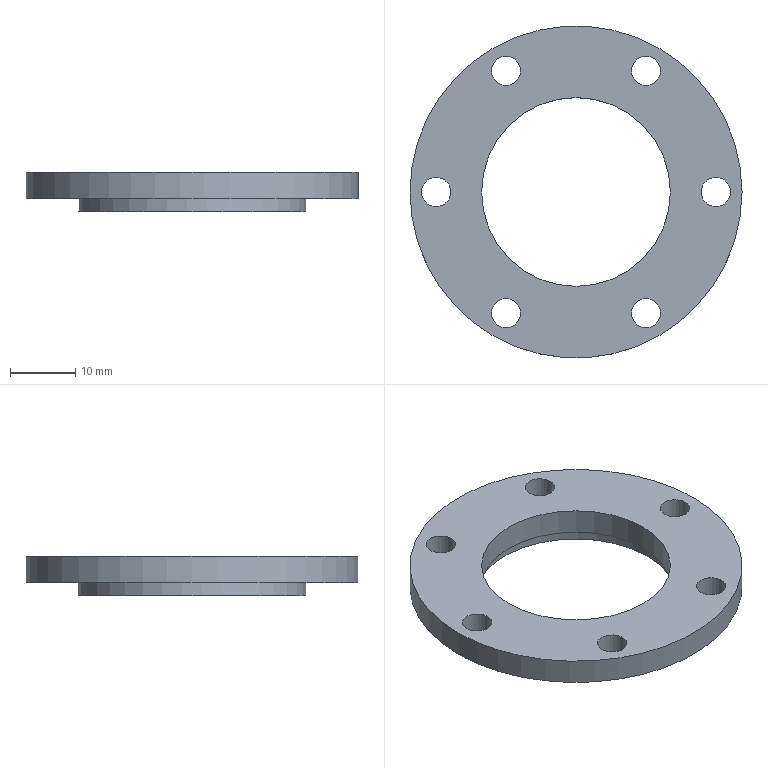Part | STEP file | zhouchenyagai3 | 1 solid | 14 faces | box 51 x 51 x 6 mm | volume 5562 mm3 | cylinder 10 | plane 4 | commonest cylinder face diameters 4.5 x6 29 x1 31 x1 35 x1 51 x1
STEP:
#1=CARTESIAN_POINT('',(0.,0.,0.));
#2=DIRECTION('',(0.,0.,1.));
#3=DIRECTION('',(1.,0.,0.));
#4=AXIS2_PLACEMENT_3D('',#1,#2,#3);
#5=CARTESIAN_POINT('',(-13.,18.62,4.));
#6=VERTEX_POINT('',#5);
#7=CARTESIAN_POINT('',(-10.75,18.62,4.));
#8=DIRECTION('',(0.,0.,-1.));
#9=DIRECTION('',(-1.,0.,0.));
#10=AXIS2_PLACEMENT_3D('',#7,#8,#9);
#11=CIRCLE('',#10,2.25);
#12=CARTESIAN_POINT('',(0.,0.,4.));
#13=DIRECTION('',(0.,0.,1.));
#14=DIRECTION('',(1.,0.,0.));
#15=AXIS2_PLACEMENT_3D('',#12,#13,#14);
#16=PLANE('',#15);
#17=CARTESIAN_POINT('',(-13.,18.62));
#18=CARTESIAN_POINT('',(-13.,22.517));
#19=CARTESIAN_POINT('',(-9.625,20.568));
#20=CARTESIAN_POINT('',(-6.25,18.62));
#21=CARTESIAN_POINT('',(-9.625,16.671));
#22=CARTESIAN_POINT('',(-13.,14.722));
#23=CARTESIAN_POINT('',(-13.,18.62));
#24=(BOUNDED_CURVE()B_SPLINE_CURVE(2,(#17,#18,#19,#20,#21,#22,#23),.UNSPECIFIED.,.T.,.F.)B_SPLINE_CURVE_WITH_KNOTS((1,2,2,2,2,1),(-2.094,0.,2.094,4.189,6.283,8.378),.UNSPECIFIED.)CURVE()GEOMETRIC_REPRESENTATION_ITEM()RATIONAL_B_SPLINE_CURVE((1.,0.5,1.,0.5,1.,0.5,1.))REPRESENTATION_ITEM(''));
#25=(GEOMETRIC_REPRESENTATION_CONTEXT(2)PARAMETRIC_REPRESENTATION_CONTEXT()REPRESENTATION_CONTEXT('',''));
#26=DEFINITIONAL_REPRESENTATION('',(#24),#25);
#27=PCURVE('',#16,#26);
#28=CARTESIAN_POINT('',(-10.75,18.62,4.));
#29=DIRECTION('',(0.,0.,-1.));
#30=DIRECTION('',(-1.,0.,0.));
#31=AXIS2_PLACEMENT_3D('',#28,#29,#30);
#32=CYLINDRICAL_SURFACE('',#31,2.25);
#33=CARTESIAN_POINT('',(0.,0.));
#34=DIRECTION('',(1.,0.));
#35=VECTOR('',#34,1.);
#36=LINE('',#33,#35);
#37=(GEOMETRIC_REPRESENTATION_CONTEXT(2)PARAMETRIC_REPRESENTATION_CONTEXT()REPRESENTATION_CONTEXT('',''));
#38=DEFINITIONAL_REPRESENTATION('',(#36),#37);
#39=PCURVE('',#32,#38);
#40=SURFACE_CURVE('',#11,(#27,#39),.PCURVE_S1.);
#41=EDGE_CURVE('',#6,#6,#40,.T.);
#42=ORIENTED_EDGE('',*,*,#41,.T.);
#43=EDGE_LOOP('',(#42));
#44=FACE_BOUND('',#43,.T.);
#45=CARTESIAN_POINT('',(19.25,0.,4.));
#46=VERTEX_POINT('',#45);
#47=CARTESIAN_POINT('',(21.5,0.,4.));
#48=DIRECTION('',(0.,0.,-1.));
#49=DIRECTION('',(-1.,0.,0.));
#50=AXIS2_PLACEMENT_3D('',#47,#48,#49);
#51=CIRCLE('',#50,2.25);
#52=CARTESIAN_POINT('',(19.25,0.));
#53=CARTESIAN_POINT('',(19.25,3.897));
#54=CARTESIAN_POINT('',(22.625,1.949));
#55=CARTESIAN_POINT('',(26.,0.));
#56=CARTESIAN_POINT('',(22.625,-1.949));
#57=CARTESIAN_POINT('',(19.25,-3.897));
#58=CARTESIAN_POINT('',(19.25,0.));
#59=(BOUNDED_CURVE()B_SPLINE_CURVE(2,(#52,#53,#54,#55,#56,#57,#58),.UNSPECIFIED.,.T.,.F.)B_SPLINE_CURVE_WITH_KNOTS((1,2,2,2,2,1),(-2.094,0.,2.094,4.189,6.283,8.378),.UNSPECIFIED.)CURVE()GEOMETRIC_REPRESENTATION_ITEM()RATIONAL_B_SPLINE_CURVE((1.,0.5,1.,0.5,1.,0.5,1.))REPRESENTATION_ITEM(''));
#60=(GEOMETRIC_REPRESENTATION_CONTEXT(2)PARAMETRIC_REPRESENTATION_CONTEXT()REPRESENTATION_CONTEXT('',''));
#61=DEFINITIONAL_REPRESENTATION('',(#59),#60);
#62=PCURVE('',#16,#61);
#63=CARTESIAN_POINT('',(21.5,0.,4.));
#64=DIRECTION('',(0.,0.,-1.));
#65=DIRECTION('',(-1.,0.,0.));
#66=AXIS2_PLACEMENT_3D('',#63,#64,#65);
#67=CYLINDRICAL_SURFACE('',#66,2.25);
#68=CARTESIAN_POINT('',(0.,0.));
#69=DIRECTION('',(1.,0.));
#70=VECTOR('',#69,1.);
#71=LINE('',#68,#70);
#72=(GEOMETRIC_REPRESENTATION_CONTEXT(2)PARAMETRIC_REPRESENTATION_CONTEXT()REPRESENTATION_CONTEXT('',''));
#73=DEFINITIONAL_REPRESENTATION('',(#71),#72);
#74=PCURVE('',#67,#73);
#75=SURFACE_CURVE('',#51,(#62,#74),.PCURVE_S1.);
#76=EDGE_CURVE('',#46,#46,#75,.T.);
#77=ORIENTED_EDGE('',*,*,#76,.T.);
#78=EDGE_LOOP('',(#77));
#79=FACE_BOUND('',#78,.T.);
#80=CARTESIAN_POINT('',(-13.,-18.62,4.));
#81=VERTEX_POINT('',#80);
#82=CARTESIAN_POINT('',(-10.75,-18.62,4.));
#83=DIRECTION('',(0.,0.,-1.));
#84=DIRECTION('',(-1.,0.,0.));
#85=AXIS2_PLACEMENT_3D('',#82,#83,#84);
#86=CIRCLE('',#85,2.25);
#87=CARTESIAN_POINT('',(-13.,-18.62));
#88=CARTESIAN_POINT('',(-13.,-14.722));
#89=CARTESIAN_POINT('',(-9.625,-16.671));
#90=CARTESIAN_POINT('',(-6.25,-18.62));
#91=CARTESIAN_POINT('',(-9.625,-20.568));
#92=CARTESIAN_POINT('',(-13.,-22.517));
#93=CARTESIAN_POINT('',(-13.,-18.62));
#94=(BOUNDED_CURVE()B_SPLINE_CURVE(2,(#87,#88,#89,#90,#91,#92,#93),.UNSPECIFIED.,.T.,.F.)B_SPLINE_CURVE_WITH_KNOTS((1,2,2,2,2,1),(-2.094,0.,2.094,4.189,6.283,8.378),.UNSPECIFIED.)CURVE()GEOMETRIC_REPRESENTATION_ITEM()RATIONAL_B_SPLINE_CURVE((1.,0.5,1.,0.5,1.,0.5,1.))REPRESENTATION_ITEM(''));
#95=(GEOMETRIC_REPRESENTATION_CONTEXT(2)PARAMETRIC_REPRESENTATION_CONTEXT()REPRESENTATION_CONTEXT('',''));
#96=DEFINITIONAL_REPRESENTATION('',(#94),#95);
#97=PCURVE('',#16,#96);
#98=CARTESIAN_POINT('',(-10.75,-18.62,4.));
#99=DIRECTION('',(0.,0.,-1.));
#100=DIRECTION('',(-1.,0.,0.));
#101=AXIS2_PLACEMENT_3D('',#98,#99,#100);
#102=CYLINDRICAL_SURFACE('',#101,2.25);
#103=CARTESIAN_POINT('',(0.,0.));
#104=DIRECTION('',(1.,0.));
#105=VECTOR('',#104,1.);
#106=LINE('',#103,#105);
#107=(GEOMETRIC_REPRESENTATION_CONTEXT(2)PARAMETRIC_REPRESENTATION_CONTEXT()REPRESENTATION_CONTEXT('',''));
#108=DEFINITIONAL_REPRESENTATION('',(#106),#107);
#109=PCURVE('',#102,#108);
#110=SURFACE_CURVE('',#86,(#97,#109),.PCURVE_S1.);
#111=EDGE_CURVE('',#81,#81,#110,.T.);
#112=ORIENTED_EDGE('',*,*,#111,.T.);
#113=EDGE_LOOP('',(#112));
#114=FACE_BOUND('',#113,.T.);
#115=CARTESIAN_POINT('',(-14.5,0.,4.));
#116=VERTEX_POINT('',#115);
#117=CARTESIAN_POINT('',(0.,0.,4.));
#118=DIRECTION('',(0.,0.,-1.));
#119=DIRECTION('',(-1.,0.,0.));
#120=AXIS2_PLACEMENT_3D('',#117,#118,#119);
#121=CIRCLE('',#120,14.5);
#122=CARTESIAN_POINT('',(-14.5,0.));
#123=CARTESIAN_POINT('',(-14.5,25.115));
#124=CARTESIAN_POINT('',(7.25,12.557));
#125=CARTESIAN_POINT('',(29.,0.));
#126=CARTESIAN_POINT('',(7.25,-12.557));
#127=CARTESIAN_POINT('',(-14.5,-25.115));
#128=CARTESIAN_POINT('',(-14.5,0.));
#129=(BOUNDED_CURVE()B_SPLINE_CURVE(2,(#122,#123,#124,#125,#126,#127,#128),.UNSPECIFIED.,.T.,.F.)B_SPLINE_CURVE_WITH_KNOTS((1,2,2,2,2,1),(-2.094,0.,2.094,4.189,6.283,8.378),.UNSPECIFIED.)CURVE()GEOMETRIC_REPRESENTATION_ITEM()RATIONAL_B_SPLINE_CURVE((1.,0.5,1.,0.5,1.,0.5,1.))REPRESENTATION_ITEM(''));
#130=(GEOMETRIC_REPRESENTATION_CONTEXT(2)PARAMETRIC_REPRESENTATION_CONTEXT()REPRESENTATION_CONTEXT('',''));
#131=DEFINITIONAL_REPRESENTATION('',(#129),#130);
#132=PCURVE('',#16,#131);
#133=CARTESIAN_POINT('',(0.,0.,4.));
#134=DIRECTION('',(0.,0.,-1.));
#135=DIRECTION('',(-1.,0.,0.));
#136=AXIS2_PLACEMENT_3D('',#133,#134,#135);
#137=CYLINDRICAL_SURFACE('',#136,14.5);
#138=CARTESIAN_POINT('',(0.,0.));
#139=DIRECTION('',(1.,0.));
#140=VECTOR('',#139,1.);
#141=LINE('',#138,#140);
#142=(GEOMETRIC_REPRESENTATION_CONTEXT(2)PARAMETRIC_REPRESENTATION_CONTEXT()REPRESENTATION_CONTEXT('',''));
#143=DEFINITIONAL_REPRESENTATION('',(#141),#142);
#144=PCURVE('',#137,#143);
#145=SURFACE_CURVE('',#121,(#132,#144),.PCURVE_S1.);
#146=EDGE_CURVE('',#116,#116,#145,.T.);
#147=ORIENTED_EDGE('',*,*,#146,.T.);
#148=EDGE_LOOP('',(#147));
#149=FACE_BOUND('',#148,.T.);
#150=CARTESIAN_POINT('',(-25.5,0.,4.));
#151=VERTEX_POINT('',#150);
#152=CARTESIAN_POINT('',(0.,0.,4.));
#153=DIRECTION('',(0.,0.,1.));
#154=DIRECTION('',(-1.,0.,0.));
#155=AXIS2_PLACEMENT_3D('',#152,#153,#154);
#156=CIRCLE('',#155,25.5);
#157=CARTESIAN_POINT('',(0.,0.));
#158=DIRECTION('',(-1.,0.));
#159=AXIS2_PLACEMENT_2D('',#157,#158);
#160=CIRCLE('',#159,25.5);
#161=(GEOMETRIC_REPRESENTATION_CONTEXT(2)PARAMETRIC_REPRESENTATION_CONTEXT()REPRESENTATION_CONTEXT('',''));
#162=DEFINITIONAL_REPRESENTATION('',(#160),#161);
#163=PCURVE('',#16,#162);
#164=CARTESIAN_POINT('',(0.,0.,4.));
#165=DIRECTION('',(0.,0.,-1.));
#166=DIRECTION('',(-1.,0.,0.));
#167=AXIS2_PLACEMENT_3D('',#164,#165,#166);
#168=CYLINDRICAL_SURFACE('',#167,25.5);
#169=CARTESIAN_POINT('',(6.283,0.));
#170=DIRECTION('',(-1.,0.));
#171=VECTOR('',#170,1.);
#172=LINE('',#169,#171);
#173=(GEOMETRIC_REPRESENTATION_CONTEXT(2)PARAMETRIC_REPRESENTATION_CONTEXT()REPRESENTATION_CONTEXT('',''));
#174=DEFINITIONAL_REPRESENTATION('',(#172),#173);
#175=PCURVE('',#168,#174);
#176=SURFACE_CURVE('',#156,(#163,#175),.PCURVE_S1.);
#177=EDGE_CURVE('',#151,#151,#176,.T.);
#178=ORIENTED_EDGE('',*,*,#177,.T.);
#179=EDGE_LOOP('',(#178));
#180=FACE_BOUND('',#179,.T.);
#181=CARTESIAN_POINT('',(-23.75,0.,4.));
#182=VERTEX_POINT('',#181);
#183=CARTESIAN_POINT('',(-21.5,0.,4.));
#184=DIRECTION('',(0.,0.,-1.));
#185=DIRECTION('',(-1.,0.,0.));
#186=AXIS2_PLACEMENT_3D('',#183,#184,#185);
#187=CIRCLE('',#186,2.25);
#188=CARTESIAN_POINT('',(-23.75,0.));
#189=CARTESIAN_POINT('',(-23.75,3.897));
#190=CARTESIAN_POINT('',(-20.375,1.949));
#191=CARTESIAN_POINT('',(-17.,0.));
#192=CARTESIAN_POINT('',(-20.375,-1.949));
#193=CARTESIAN_POINT('',(-23.75,-3.897));
#194=CARTESIAN_POINT('',(-23.75,0.));
#195=(BOUNDED_CURVE()B_SPLINE_CURVE(2,(#188,#189,#190,#191,#192,#193,#194),.UNSPECIFIED.,.T.,.F.)B_SPLINE_CURVE_WITH_KNOTS((1,2,2,2,2,1),(-2.094,0.,2.094,4.189,6.283,8.378),.UNSPECIFIED.)CURVE()GEOMETRIC_REPRESENTATION_ITEM()RATIONAL_B_SPLINE_CURVE((1.,0.5,1.,0.5,1.,0.5,1.))REPRESENTATION_ITEM(''));
#196=(GEOMETRIC_REPRESENTATION_CONTEXT(2)PARAMETRIC_REPRESENTATION_CONTEXT()REPRESENTATION_CONTEXT('',''));
#197=DEFINITIONAL_REPRESENTATION('',(#195),#196);
#198=PCURVE('',#16,#197);
#199=CARTESIAN_POINT('',(-21.5,0.,4.));
#200=DIRECTION('',(0.,0.,-1.));
#201=DIRECTION('',(-1.,0.,0.));
#202=AXIS2_PLACEMENT_3D('',#199,#200,#201);
#203=CYLINDRICAL_SURFACE('',#202,2.25);
#204=CARTESIAN_POINT('',(0.,0.));
#205=DIRECTION('',(1.,0.));
#206=VECTOR('',#205,1.);
#207=LINE('',#204,#206);
#208=(GEOMETRIC_REPRESENTATION_CONTEXT(2)PARAMETRIC_REPRESENTATION_CONTEXT()REPRESENTATION_CONTEXT('',''));
#209=DEFINITIONAL_REPRESENTATION('',(#207),#208);
#210=PCURVE('',#203,#209);
#211=SURFACE_CURVE('',#187,(#198,#210),.PCURVE_S1.);
#212=EDGE_CURVE('',#182,#182,#211,.T.);
#213=ORIENTED_EDGE('',*,*,#212,.T.);
#214=EDGE_LOOP('',(#213));
#215=FACE_BOUND('',#214,.T.);
#216=CARTESIAN_POINT('',(8.5,-18.62,4.));
#217=VERTEX_POINT('',#216);
#218=CARTESIAN_POINT('',(10.75,-18.62,4.));
#219=DIRECTION('',(0.,0.,-1.));
#220=DIRECTION('',(-1.,0.,0.));
#221=AXIS2_PLACEMENT_3D('',#218,#219,#220);
#222=CIRCLE('',#221,2.25);
#223=CARTESIAN_POINT('',(8.5,-18.62));
#224=CARTESIAN_POINT('',(8.5,-14.722));
#225=CARTESIAN_POINT('',(11.875,-16.671));
#226=CARTESIAN_POINT('',(15.25,-18.62));
#227=CARTESIAN_POINT('',(11.875,-20.568));
#228=CARTESIAN_POINT('',(8.5,-22.517));
#229=CARTESIAN_POINT('',(8.5,-18.62));
#230=(BOUNDED_CURVE()B_SPLINE_CURVE(2,(#223,#224,#225,#226,#227,#228,#229),.UNSPECIFIED.,.T.,.F.)B_SPLINE_CURVE_WITH_KNOTS((1,2,2,2,2,1),(-2.094,0.,2.094,4.189,6.283,8.378),.UNSPECIFIED.)CURVE()GEOMETRIC_REPRESENTATION_ITEM()RATIONAL_B_SPLINE_CURVE((1.,0.5,1.,0.5,1.,0.5,1.))REPRESENTATION_ITEM(''));
#231=(GEOMETRIC_REPRESENTATION_CONTEXT(2)PARAMETRIC_REPRESENTATION_CONTEXT()REPRESENTATION_CONTEXT('',''));
#232=DEFINITIONAL_REPRESENTATION('',(#230),#231);
#233=PCURVE('',#16,#232);
#234=CARTESIAN_POINT('',(10.75,-18.62,4.));
#235=DIRECTION('',(0.,0.,-1.));
#236=DIRECTION('',(-1.,0.,0.));
#237=AXIS2_PLACEMENT_3D('',#234,#235,#236);
#238=CYLINDRICAL_SURFACE('',#237,2.25);
#239=CARTESIAN_POINT('',(0.,0.));
#240=DIRECTION('',(1.,0.));
#241=VECTOR('',#240,1.);
#242=LINE('',#239,#241);
#243=(GEOMETRIC_REPRESENTATION_CONTEXT(2)PARAMETRIC_REPRESENTATION_CONTEXT()REPRESENTATION_CONTEXT('',''));
#244=DEFINITIONAL_REPRESENTATION('',(#242),#243);
#245=PCURVE('',#238,#244);
#246=SURFACE_CURVE('',#222,(#233,#245),.PCURVE_S1.);
#247=EDGE_CURVE('',#217,#217,#246,.T.);
#248=ORIENTED_EDGE('',*,*,#247,.T.);
#249=EDGE_LOOP('',(#248));
#250=FACE_BOUND('',#249,.T.);
#251=CARTESIAN_POINT('',(8.5,18.62,4.));
#252=VERTEX_POINT('',#251);
#253=CARTESIAN_POINT('',(10.75,18.62,4.));
#254=DIRECTION('',(0.,0.,-1.));
#255=DIRECTION('',(-1.,0.,0.));
#256=AXIS2_PLACEMENT_3D('',#253,#254,#255);
#257=CIRCLE('',#256,2.25);
#258=CARTESIAN_POINT('',(8.5,18.62));
#259=CARTESIAN_POINT('',(8.5,22.517));
#260=CARTESIAN_POINT('',(11.875,20.568));
#261=CARTESIAN_POINT('',(15.25,18.62));
#262=CARTESIAN_POINT('',(11.875,16.671));
#263=CARTESIAN_POINT('',(8.5,14.722));
#264=CARTESIAN_POINT('',(8.5,18.62));
#265=(BOUNDED_CURVE()B_SPLINE_CURVE(2,(#258,#259,#260,#261,#262,#263,#264),.UNSPECIFIED.,.T.,.F.)B_SPLINE_CURVE_WITH_KNOTS((1,2,2,2,2,1),(-2.094,0.,2.094,4.189,6.283,8.378),.UNSPECIFIED.)CURVE()GEOMETRIC_REPRESENTATION_ITEM()RATIONAL_B_SPLINE_CURVE((1.,0.5,1.,0.5,1.,0.5,1.))REPRESENTATION_ITEM(''));
#266=(GEOMETRIC_REPRESENTATION_CONTEXT(2)PARAMETRIC_REPRESENTATION_CONTEXT()REPRESENTATION_CONTEXT('',''));
#267=DEFINITIONAL_REPRESENTATION('',(#265),#266);
#268=PCURVE('',#16,#267);
#269=CARTESIAN_POINT('',(10.75,18.62,4.));
#270=DIRECTION('',(0.,0.,-1.));
#271=DIRECTION('',(-1.,0.,0.));
#272=AXIS2_PLACEMENT_3D('',#269,#270,#271);
#273=CYLINDRICAL_SURFACE('',#272,2.25);
#274=CARTESIAN_POINT('',(0.,0.));
#275=DIRECTION('',(1.,0.));
#276=VECTOR('',#275,1.);
#277=LINE('',#274,#276);
#278=(GEOMETRIC_REPRESENTATION_CONTEXT(2)PARAMETRIC_REPRESENTATION_CONTEXT()REPRESENTATION_CONTEXT('',''));
#279=DEFINITIONAL_REPRESENTATION('',(#277),#278);
#280=PCURVE('',#273,#279);
#281=SURFACE_CURVE('',#257,(#268,#280),.PCURVE_S1.);
#282=EDGE_CURVE('',#252,#252,#281,.T.);
#283=ORIENTED_EDGE('',*,*,#282,.T.);
#284=EDGE_LOOP('',(#283));
#285=FACE_BOUND('',#284,.T.);
#286=ADVANCED_FACE('',(#44,#79,#114,#149,#180,#215,#250,#285),#16,.T.);
#287=ORIENTED_EDGE('',*,*,#41,.T.);
#288=CARTESIAN_POINT('',(-13.,18.62,0.));
#289=VERTEX_POINT('',#288);
#290=CARTESIAN_POINT('',(-13.,18.62,4.));
#291=CARTESIAN_POINT('',(-13.,18.62,0.));
#292=B_SPLINE_CURVE_WITH_KNOTS('',1,(#290,#291),.UNSPECIFIED.,.F.,.F.,(2,2),(0.,4.),.PIECEWISE_BEZIER_KNOTS.);
#293=CARTESIAN_POINT('',(6.283,0.));
#294=DIRECTION('',(0.,1.));
#295=VECTOR('',#294,1.);
#296=LINE('',#293,#295);
#297=(GEOMETRIC_REPRESENTATION_CONTEXT(2)PARAMETRIC_REPRESENTATION_CONTEXT()REPRESENTATION_CONTEXT('',''));
#298=DEFINITIONAL_REPRESENTATION('',(#296),#297);
#299=PCURVE('',#32,#298);
#300=CARTESIAN_POINT('',(0.,0.));
#301=DIRECTION('',(0.,1.));
#302=VECTOR('',#301,1.);
#303=LINE('',#300,#302);
#304=(GEOMETRIC_REPRESENTATION_CONTEXT(2)PARAMETRIC_REPRESENTATION_CONTEXT()REPRESENTATION_CONTEXT('',''));
#305=DEFINITIONAL_REPRESENTATION('',(#303),#304);
#306=PCURVE('',#32,#305);
#307=SEAM_CURVE('',#292,(#299,#306),.PCURVE_S1.);
#308=EDGE_CURVE('',#6,#289,#307,.T.);
#309=ORIENTED_EDGE('',*,*,#308,.T.);
#310=CARTESIAN_POINT('',(-10.75,18.62,0.));
#311=DIRECTION('',(0.,0.,1.));
#312=DIRECTION('',(-1.,0.,0.));
#313=AXIS2_PLACEMENT_3D('',#310,#311,#312);
#314=CIRCLE('',#313,2.25);
#315=CARTESIAN_POINT('',(6.283,4.));
#316=DIRECTION('',(-1.,0.));
#317=VECTOR('',#316,1.);
#318=LINE('',#315,#317);
#319=(GEOMETRIC_REPRESENTATION_CONTEXT(2)PARAMETRIC_REPRESENTATION_CONTEXT()REPRESENTATION_CONTEXT('',''));
#320=DEFINITIONAL_REPRESENTATION('',(#318),#319);
#321=PCURVE('',#32,#320);
#322=CARTESIAN_POINT('',(0.,0.,0.));
#323=DIRECTION('',(0.,0.,1.));
#324=DIRECTION('',(1.,0.,0.));
#325=AXIS2_PLACEMENT_3D('',#322,#323,#324);
#326=PLANE('',#325);
#327=CARTESIAN_POINT('',(-10.75,18.62));
#328=DIRECTION('',(-1.,0.));
#329=AXIS2_PLACEMENT_2D('',#327,#328);
#330=CIRCLE('',#329,2.25);
#331=(GEOMETRIC_REPRESENTATION_CONTEXT(2)PARAMETRIC_REPRESENTATION_CONTEXT()REPRESENTATION_CONTEXT('',''));
#332=DEFINITIONAL_REPRESENTATION('',(#330),#331);
#333=PCURVE('',#326,#332);
#334=SURFACE_CURVE('',#314,(#321,#333),.PCURVE_S1.);
#335=EDGE_CURVE('',#289,#289,#334,.T.);
#336=ORIENTED_EDGE('',*,*,#335,.T.);
#337=ORIENTED_EDGE('',*,*,#308,.F.);
#338=EDGE_LOOP('',(#287,#309,#336,#337));
#339=FACE_BOUND('',#338,.F.);
#340=ADVANCED_FACE('',(#339),#32,.F.);
#341=ORIENTED_EDGE('',*,*,#76,.T.);
#342=CARTESIAN_POINT('',(19.25,0.,0.));
#343=VERTEX_POINT('',#342);
#344=CARTESIAN_POINT('',(19.25,0.,4.));
#345=CARTESIAN_POINT('',(19.25,0.,0.));
#346=B_SPLINE_CURVE_WITH_KNOTS('',1,(#344,#345),.UNSPECIFIED.,.F.,.F.,(2,2),(0.,4.),.PIECEWISE_BEZIER_KNOTS.);
#347=CARTESIAN_POINT('',(6.283,0.));
#348=DIRECTION('',(0.,1.));
#349=VECTOR('',#348,1.);
#350=LINE('',#347,#349);
#351=(GEOMETRIC_REPRESENTATION_CONTEXT(2)PARAMETRIC_REPRESENTATION_CONTEXT()REPRESENTATION_CONTEXT('',''));
#352=DEFINITIONAL_REPRESENTATION('',(#350),#351);
#353=PCURVE('',#67,#352);
#354=CARTESIAN_POINT('',(0.,0.));
#355=DIRECTION('',(0.,1.));
#356=VECTOR('',#355,1.);
#357=LINE('',#354,#356);
#358=(GEOMETRIC_REPRESENTATION_CONTEXT(2)PARAMETRIC_REPRESENTATION_CONTEXT()REPRESENTATION_CONTEXT('',''));
#359=DEFINITIONAL_REPRESENTATION('',(#357),#358);
#360=PCURVE('',#67,#359);
#361=SEAM_CURVE('',#346,(#353,#360),.PCURVE_S1.);
#362=EDGE_CURVE('',#46,#343,#361,.T.);
#363=ORIENTED_EDGE('',*,*,#362,.T.);
#364=CARTESIAN_POINT('',(21.5,0.,0.));
#365=DIRECTION('',(0.,0.,1.));
#366=DIRECTION('',(-1.,0.,0.));
#367=AXIS2_PLACEMENT_3D('',#364,#365,#366);
#368=CIRCLE('',#367,2.25);
#369=CARTESIAN_POINT('',(6.283,4.));
#370=DIRECTION('',(-1.,0.));
#371=VECTOR('',#370,1.);
#372=LINE('',#369,#371);
#373=(GEOMETRIC_REPRESENTATION_CONTEXT(2)PARAMETRIC_REPRESENTATION_CONTEXT()REPRESENTATION_CONTEXT('',''));
#374=DEFINITIONAL_REPRESENTATION('',(#372),#373);
#375=PCURVE('',#67,#374);
#376=CARTESIAN_POINT('',(21.5,0.));
#377=DIRECTION('',(-1.,0.));
#378=AXIS2_PLACEMENT_2D('',#376,#377);
#379=CIRCLE('',#378,2.25);
#380=(GEOMETRIC_REPRESENTATION_CONTEXT(2)PARAMETRIC_REPRESENTATION_CONTEXT()REPRESENTATION_CONTEXT('',''));
#381=DEFINITIONAL_REPRESENTATION('',(#379),#380);
#382=PCURVE('',#326,#381);
#383=SURFACE_CURVE('',#368,(#375,#382),.PCURVE_S1.);
#384=EDGE_CURVE('',#343,#343,#383,.T.);
#385=ORIENTED_EDGE('',*,*,#384,.T.);
#386=ORIENTED_EDGE('',*,*,#362,.F.);
#387=EDGE_LOOP('',(#341,#363,#385,#386));
#388=FACE_BOUND('',#387,.F.);
#389=ADVANCED_FACE('',(#388),#67,.F.);
#390=ORIENTED_EDGE('',*,*,#111,.T.);
#391=CARTESIAN_POINT('',(-13.,-18.62,0.));
#392=VERTEX_POINT('',#391);
#393=CARTESIAN_POINT('',(-13.,-18.62,4.));
#394=CARTESIAN_POINT('',(-13.,-18.62,0.));
#395=B_SPLINE_CURVE_WITH_KNOTS('',1,(#393,#394),.UNSPECIFIED.,.F.,.F.,(2,2),(0.,4.),.PIECEWISE_BEZIER_KNOTS.);
#396=CARTESIAN_POINT('',(6.283,0.));
#397=DIRECTION('',(0.,1.));
#398=VECTOR('',#397,1.);
#399=LINE('',#396,#398);
#400=(GEOMETRIC_REPRESENTATION_CONTEXT(2)PARAMETRIC_REPRESENTATION_CONTEXT()REPRESENTATION_CONTEXT('',''));
#401=DEFINITIONAL_REPRESENTATION('',(#399),#400);
#402=PCURVE('',#102,#401);
#403=CARTESIAN_POINT('',(0.,0.));
#404=DIRECTION('',(0.,1.));
#405=VECTOR('',#404,1.);
#406=LINE('',#403,#405);
#407=(GEOMETRIC_REPRESENTATION_CONTEXT(2)PARAMETRIC_REPRESENTATION_CONTEXT()REPRESENTATION_CONTEXT('',''));
#408=DEFINITIONAL_REPRESENTATION('',(#406),#407);
#409=PCURVE('',#102,#408);
#410=SEAM_CURVE('',#395,(#402,#409),.PCURVE_S1.);
#411=EDGE_CURVE('',#81,#392,#410,.T.);
#412=ORIENTED_EDGE('',*,*,#411,.T.);
#413=CARTESIAN_POINT('',(-10.75,-18.62,0.));
#414=DIRECTION('',(0.,0.,1.));
#415=DIRECTION('',(-1.,0.,0.));
#416=AXIS2_PLACEMENT_3D('',#413,#414,#415);
#417=CIRCLE('',#416,2.25);
#418=CARTESIAN_POINT('',(6.283,4.));
#419=DIRECTION('',(-1.,0.));
#420=VECTOR('',#419,1.);
#421=LINE('',#418,#420);
#422=(GEOMETRIC_REPRESENTATION_CONTEXT(2)PARAMETRIC_REPRESENTATION_CONTEXT()REPRESENTATION_CONTEXT('',''));
#423=DEFINITIONAL_REPRESENTATION('',(#421),#422);
#424=PCURVE('',#102,#423);
#425=CARTESIAN_POINT('',(-10.75,-18.62));
#426=DIRECTION('',(-1.,0.));
#427=AXIS2_PLACEMENT_2D('',#425,#426);
#428=CIRCLE('',#427,2.25);
#429=(GEOMETRIC_REPRESENTATION_CONTEXT(2)PARAMETRIC_REPRESENTATION_CONTEXT()REPRESENTATION_CONTEXT('',''));
#430=DEFINITIONAL_REPRESENTATION('',(#428),#429);
#431=PCURVE('',#326,#430);
#432=SURFACE_CURVE('',#417,(#424,#431),.PCURVE_S1.);
#433=EDGE_CURVE('',#392,#392,#432,.T.);
#434=ORIENTED_EDGE('',*,*,#433,.T.);
#435=ORIENTED_EDGE('',*,*,#411,.F.);
#436=EDGE_LOOP('',(#390,#412,#434,#435));
#437=FACE_BOUND('',#436,.F.);
#438=ADVANCED_FACE('',(#437),#102,.F.);
#439=ORIENTED_EDGE('',*,*,#146,.T.);
#440=CARTESIAN_POINT('',(-14.5,0.,0.));
#441=VERTEX_POINT('',#440);
#442=CARTESIAN_POINT('',(-14.5,0.,4.));
#443=CARTESIAN_POINT('',(-14.5,0.,0.));
#444=B_SPLINE_CURVE_WITH_KNOTS('',1,(#442,#443),.UNSPECIFIED.,.F.,.F.,(2,2),(0.,4.),.PIECEWISE_BEZIER_KNOTS.);
#445=CARTESIAN_POINT('',(6.283,0.));
#446=DIRECTION('',(0.,1.));
#447=VECTOR('',#446,1.);
#448=LINE('',#445,#447);
#449=(GEOMETRIC_REPRESENTATION_CONTEXT(2)PARAMETRIC_REPRESENTATION_CONTEXT()REPRESENTATION_CONTEXT('',''));
#450=DEFINITIONAL_REPRESENTATION('',(#448),#449);
#451=PCURVE('',#137,#450);
#452=CARTESIAN_POINT('',(0.,0.));
#453=DIRECTION('',(0.,1.));
#454=VECTOR('',#453,1.);
#455=LINE('',#452,#454);
#456=(GEOMETRIC_REPRESENTATION_CONTEXT(2)PARAMETRIC_REPRESENTATION_CONTEXT()REPRESENTATION_CONTEXT('',''));
#457=DEFINITIONAL_REPRESENTATION('',(#455),#456);
#458=PCURVE('',#137,#457);
#459=SEAM_CURVE('',#444,(#451,#458),.PCURVE_S1.);
#460=EDGE_CURVE('',#116,#441,#459,.T.);
#461=ORIENTED_EDGE('',*,*,#460,.T.);
#462=CARTESIAN_POINT('',(0.,0.,0.));
#463=DIRECTION('',(0.,0.,1.));
#464=DIRECTION('',(-1.,0.,0.));
#465=AXIS2_PLACEMENT_3D('',#462,#463,#464);
#466=CIRCLE('',#465,14.5);
#467=CARTESIAN_POINT('',(6.283,4.));
#468=DIRECTION('',(-1.,0.));
#469=VECTOR('',#468,1.);
#470=LINE('',#467,#469);
#471=(GEOMETRIC_REPRESENTATION_CONTEXT(2)PARAMETRIC_REPRESENTATION_CONTEXT()REPRESENTATION_CONTEXT('',''));
#472=DEFINITIONAL_REPRESENTATION('',(#470),#471);
#473=PCURVE('',#137,#472);
#474=CARTESIAN_POINT('',(0.,0.,0.));
#475=DIRECTION('',(0.,0.,1.));
#476=DIRECTION('',(1.,0.,0.));
#477=AXIS2_PLACEMENT_3D('',#474,#475,#476);
#478=PLANE('',#477);
#479=CARTESIAN_POINT('',(0.,0.));
#480=DIRECTION('',(-1.,0.));
#481=AXIS2_PLACEMENT_2D('',#479,#480);
#482=CIRCLE('',#481,14.5);
#483=(GEOMETRIC_REPRESENTATION_CONTEXT(2)PARAMETRIC_REPRESENTATION_CONTEXT()REPRESENTATION_CONTEXT('',''));
#484=DEFINITIONAL_REPRESENTATION('',(#482),#483);
#485=PCURVE('',#478,#484);
#486=SURFACE_CURVE('',#466,(#473,#485),.PCURVE_S1.);
#487=EDGE_CURVE('',#441,#441,#486,.T.);
#488=ORIENTED_EDGE('',*,*,#487,.T.);
#489=ORIENTED_EDGE('',*,*,#460,.F.);
#490=EDGE_LOOP('',(#439,#461,#488,#489));
#491=FACE_BOUND('',#490,.F.);
#492=ADVANCED_FACE('',(#491),#137,.F.);
#493=CARTESIAN_POINT('',(-25.5,0.,0.));
#494=VERTEX_POINT('',#493);
#495=CARTESIAN_POINT('',(0.,0.,0.));
#496=DIRECTION('',(0.,0.,1.));
#497=DIRECTION('',(-1.,0.,0.));
#498=AXIS2_PLACEMENT_3D('',#495,#496,#497);
#499=CIRCLE('',#498,25.5);
#500=CARTESIAN_POINT('',(6.283,4.));
#501=DIRECTION('',(-1.,0.));
#502=VECTOR('',#501,1.);
#503=LINE('',#500,#502);
#504=(GEOMETRIC_REPRESENTATION_CONTEXT(2)PARAMETRIC_REPRESENTATION_CONTEXT()REPRESENTATION_CONTEXT('',''));
#505=DEFINITIONAL_REPRESENTATION('',(#503),#504);
#506=PCURVE('',#168,#505);
#507=CARTESIAN_POINT('',(0.,0.));
#508=DIRECTION('',(-1.,0.));
#509=AXIS2_PLACEMENT_2D('',#507,#508);
#510=CIRCLE('',#509,25.5);
#511=(GEOMETRIC_REPRESENTATION_CONTEXT(2)PARAMETRIC_REPRESENTATION_CONTEXT()REPRESENTATION_CONTEXT('',''));
#512=DEFINITIONAL_REPRESENTATION('',(#510),#511);
#513=PCURVE('',#326,#512);
#514=SURFACE_CURVE('',#499,(#506,#513),.PCURVE_S1.);
#515=EDGE_CURVE('',#494,#494,#514,.T.);
#516=ORIENTED_EDGE('',*,*,#515,.T.);
#517=CARTESIAN_POINT('',(-25.5,0.,4.));
#518=CARTESIAN_POINT('',(-25.5,0.,0.));
#519=B_SPLINE_CURVE_WITH_KNOTS('',1,(#517,#518),.UNSPECIFIED.,.F.,.F.,(2,2),(0.,4.),.PIECEWISE_BEZIER_KNOTS.);
#520=CARTESIAN_POINT('',(0.,0.));
#521=DIRECTION('',(0.,1.));
#522=VECTOR('',#521,1.);
#523=LINE('',#520,#522);
#524=(GEOMETRIC_REPRESENTATION_CONTEXT(2)PARAMETRIC_REPRESENTATION_CONTEXT()REPRESENTATION_CONTEXT('',''));
#525=DEFINITIONAL_REPRESENTATION('',(#523),#524);
#526=PCURVE('',#168,#525);
#527=CARTESIAN_POINT('',(6.283,0.));
#528=DIRECTION('',(0.,1.));
#529=VECTOR('',#528,1.);
#530=LINE('',#527,#529);
#531=(GEOMETRIC_REPRESENTATION_CONTEXT(2)PARAMETRIC_REPRESENTATION_CONTEXT()REPRESENTATION_CONTEXT('',''));
#532=DEFINITIONAL_REPRESENTATION('',(#530),#531);
#533=PCURVE('',#168,#532);
#534=SEAM_CURVE('',#519,(#526,#533),.PCURVE_S1.);
#535=EDGE_CURVE('',#151,#494,#534,.T.);
#536=ORIENTED_EDGE('',*,*,#535,.F.);
#537=ORIENTED_EDGE('',*,*,#177,.F.);
#538=ORIENTED_EDGE('',*,*,#535,.T.);
#539=EDGE_LOOP('',(#516,#536,#537,#538));
#540=FACE_BOUND('',#539,.T.);
#541=ADVANCED_FACE('',(#540),#168,.T.);
#542=ORIENTED_EDGE('',*,*,#212,.T.);
#543=CARTESIAN_POINT('',(-23.75,0.,0.));
#544=VERTEX_POINT('',#543);
#545=CARTESIAN_POINT('',(-23.75,0.,4.));
#546=CARTESIAN_POINT('',(-23.75,0.,0.));
#547=B_SPLINE_CURVE_WITH_KNOTS('',1,(#545,#546),.UNSPECIFIED.,.F.,.F.,(2,2),(0.,4.),.PIECEWISE_BEZIER_KNOTS.);
#548=CARTESIAN_POINT('',(6.283,0.));
#549=DIRECTION('',(0.,1.));
#550=VECTOR('',#549,1.);
#551=LINE('',#548,#550);
#552=(GEOMETRIC_REPRESENTATION_CONTEXT(2)PARAMETRIC_REPRESENTATION_CONTEXT()REPRESENTATION_CONTEXT('',''));
#553=DEFINITIONAL_REPRESENTATION('',(#551),#552);
#554=PCURVE('',#203,#553);
#555=CARTESIAN_POINT('',(0.,0.));
#556=DIRECTION('',(0.,1.));
#557=VECTOR('',#556,1.);
#558=LINE('',#555,#557);
#559=(GEOMETRIC_REPRESENTATION_CONTEXT(2)PARAMETRIC_REPRESENTATION_CONTEXT()REPRESENTATION_CONTEXT('',''));
#560=DEFINITIONAL_REPRESENTATION('',(#558),#559);
#561=PCURVE('',#203,#560);
#562=SEAM_CURVE('',#547,(#554,#561),.PCURVE_S1.);
#563=EDGE_CURVE('',#182,#544,#562,.T.);
#564=ORIENTED_EDGE('',*,*,#563,.T.);
#565=CARTESIAN_POINT('',(-21.5,0.,0.));
#566=DIRECTION('',(0.,0.,1.));
#567=DIRECTION('',(-1.,0.,0.));
#568=AXIS2_PLACEMENT_3D('',#565,#566,#567);
#569=CIRCLE('',#568,2.25);
#570=CARTESIAN_POINT('',(6.283,4.));
#571=DIRECTION('',(-1.,0.));
#572=VECTOR('',#571,1.);
#573=LINE('',#570,#572);
#574=(GEOMETRIC_REPRESENTATION_CONTEXT(2)PARAMETRIC_REPRESENTATION_CONTEXT()REPRESENTATION_CONTEXT('',''));
#575=DEFINITIONAL_REPRESENTATION('',(#573),#574);
#576=PCURVE('',#203,#575);
#577=CARTESIAN_POINT('',(-21.5,0.));
#578=DIRECTION('',(-1.,0.));
#579=AXIS2_PLACEMENT_2D('',#577,#578);
#580=CIRCLE('',#579,2.25);
#581=(GEOMETRIC_REPRESENTATION_CONTEXT(2)PARAMETRIC_REPRESENTATION_CONTEXT()REPRESENTATION_CONTEXT('',''));
#582=DEFINITIONAL_REPRESENTATION('',(#580),#581);
#583=PCURVE('',#326,#582);
#584=SURFACE_CURVE('',#569,(#576,#583),.PCURVE_S1.);
#585=EDGE_CURVE('',#544,#544,#584,.T.);
#586=ORIENTED_EDGE('',*,*,#585,.T.);
#587=ORIENTED_EDGE('',*,*,#563,.F.);
#588=EDGE_LOOP('',(#542,#564,#586,#587));
#589=FACE_BOUND('',#588,.F.);
#590=ADVANCED_FACE('',(#589),#203,.F.);
#591=ORIENTED_EDGE('',*,*,#247,.T.);
#592=CARTESIAN_POINT('',(8.5,-18.62,0.));
#593=VERTEX_POINT('',#592);
#594=CARTESIAN_POINT('',(8.5,-18.62,4.));
#595=CARTESIAN_POINT('',(8.5,-18.62,0.));
#596=B_SPLINE_CURVE_WITH_KNOTS('',1,(#594,#595),.UNSPECIFIED.,.F.,.F.,(2,2),(0.,4.),.PIECEWISE_BEZIER_KNOTS.);
#597=CARTESIAN_POINT('',(6.283,0.));
#598=DIRECTION('',(0.,1.));
#599=VECTOR('',#598,1.);
#600=LINE('',#597,#599);
#601=(GEOMETRIC_REPRESENTATION_CONTEXT(2)PARAMETRIC_REPRESENTATION_CONTEXT()REPRESENTATION_CONTEXT('',''));
#602=DEFINITIONAL_REPRESENTATION('',(#600),#601);
#603=PCURVE('',#238,#602);
#604=CARTESIAN_POINT('',(0.,0.));
#605=DIRECTION('',(0.,1.));
#606=VECTOR('',#605,1.);
#607=LINE('',#604,#606);
#608=(GEOMETRIC_REPRESENTATION_CONTEXT(2)PARAMETRIC_REPRESENTATION_CONTEXT()REPRESENTATION_CONTEXT('',''));
#609=DEFINITIONAL_REPRESENTATION('',(#607),#608);
#610=PCURVE('',#238,#609);
#611=SEAM_CURVE('',#596,(#603,#610),.PCURVE_S1.);
#612=EDGE_CURVE('',#217,#593,#611,.T.);
#613=ORIENTED_EDGE('',*,*,#612,.T.);
#614=CARTESIAN_POINT('',(10.75,-18.62,0.));
#615=DIRECTION('',(0.,0.,1.));
#616=DIRECTION('',(-1.,0.,0.));
#617=AXIS2_PLACEMENT_3D('',#614,#615,#616);
#618=CIRCLE('',#617,2.25);
#619=CARTESIAN_POINT('',(6.283,4.));
#620=DIRECTION('',(-1.,0.));
#621=VECTOR('',#620,1.);
#622=LINE('',#619,#621);
#623=(GEOMETRIC_REPRESENTATION_CONTEXT(2)PARAMETRIC_REPRESENTATION_CONTEXT()REPRESENTATION_CONTEXT('',''));
#624=DEFINITIONAL_REPRESENTATION('',(#622),#623);
#625=PCURVE('',#238,#624);
#626=CARTESIAN_POINT('',(10.75,-18.62));
#627=DIRECTION('',(-1.,0.));
#628=AXIS2_PLACEMENT_2D('',#626,#627);
#629=CIRCLE('',#628,2.25);
#630=(GEOMETRIC_REPRESENTATION_CONTEXT(2)PARAMETRIC_REPRESENTATION_CONTEXT()REPRESENTATION_CONTEXT('',''));
#631=DEFINITIONAL_REPRESENTATION('',(#629),#630);
#632=PCURVE('',#326,#631);
#633=SURFACE_CURVE('',#618,(#625,#632),.PCURVE_S1.);
#634=EDGE_CURVE('',#593,#593,#633,.T.);
#635=ORIENTED_EDGE('',*,*,#634,.T.);
#636=ORIENTED_EDGE('',*,*,#612,.F.);
#637=EDGE_LOOP('',(#591,#613,#635,#636));
#638=FACE_BOUND('',#637,.F.);
#639=ADVANCED_FACE('',(#638),#238,.F.);
#640=ORIENTED_EDGE('',*,*,#282,.T.);
#641=CARTESIAN_POINT('',(8.5,18.62,0.));
#642=VERTEX_POINT('',#641);
#643=CARTESIAN_POINT('',(8.5,18.62,4.));
#644=CARTESIAN_POINT('',(8.5,18.62,0.));
#645=B_SPLINE_CURVE_WITH_KNOTS('',1,(#643,#644),.UNSPECIFIED.,.F.,.F.,(2,2),(0.,4.),.PIECEWISE_BEZIER_KNOTS.);
#646=CARTESIAN_POINT('',(6.283,0.));
#647=DIRECTION('',(0.,1.));
#648=VECTOR('',#647,1.);
#649=LINE('',#646,#648);
#650=(GEOMETRIC_REPRESENTATION_CONTEXT(2)PARAMETRIC_REPRESENTATION_CONTEXT()REPRESENTATION_CONTEXT('',''));
#651=DEFINITIONAL_REPRESENTATION('',(#649),#650);
#652=PCURVE('',#273,#651);
#653=CARTESIAN_POINT('',(0.,0.));
#654=DIRECTION('',(0.,1.));
#655=VECTOR('',#654,1.);
#656=LINE('',#653,#655);
#657=(GEOMETRIC_REPRESENTATION_CONTEXT(2)PARAMETRIC_REPRESENTATION_CONTEXT()REPRESENTATION_CONTEXT('',''));
#658=DEFINITIONAL_REPRESENTATION('',(#656),#657);
#659=PCURVE('',#273,#658);
#660=SEAM_CURVE('',#645,(#652,#659),.PCURVE_S1.);
#661=EDGE_CURVE('',#252,#642,#660,.T.);
#662=ORIENTED_EDGE('',*,*,#661,.T.);
#663=CARTESIAN_POINT('',(10.75,18.62,0.));
#664=DIRECTION('',(0.,0.,1.));
#665=DIRECTION('',(-1.,0.,0.));
#666=AXIS2_PLACEMENT_3D('',#663,#664,#665);
#667=CIRCLE('',#666,2.25);
#668=CARTESIAN_POINT('',(6.283,4.));
#669=DIRECTION('',(-1.,0.));
#670=VECTOR('',#669,1.);
#671=LINE('',#668,#670);
#672=(GEOMETRIC_REPRESENTATION_CONTEXT(2)PARAMETRIC_REPRESENTATION_CONTEXT()REPRESENTATION_CONTEXT('',''));
#673=DEFINITIONAL_REPRESENTATION('',(#671),#672);
#674=PCURVE('',#273,#673);
#675=CARTESIAN_POINT('',(10.75,18.62));
#676=DIRECTION('',(-1.,0.));
#677=AXIS2_PLACEMENT_2D('',#675,#676);
#678=CIRCLE('',#677,2.25);
#679=(GEOMETRIC_REPRESENTATION_CONTEXT(2)PARAMETRIC_REPRESENTATION_CONTEXT()REPRESENTATION_CONTEXT('',''));
#680=DEFINITIONAL_REPRESENTATION('',(#678),#679);
#681=PCURVE('',#326,#680);
#682=SURFACE_CURVE('',#667,(#674,#681),.PCURVE_S1.);
#683=EDGE_CURVE('',#642,#642,#682,.T.);
#684=ORIENTED_EDGE('',*,*,#683,.T.);
#685=ORIENTED_EDGE('',*,*,#661,.F.);
#686=EDGE_LOOP('',(#640,#662,#684,#685));
#687=FACE_BOUND('',#686,.F.);
#688=ADVANCED_FACE('',(#687),#273,.F.);
#689=ORIENTED_EDGE('',*,*,#335,.T.);
#690=EDGE_LOOP('',(#689));
#691=FACE_BOUND('',#690,.T.);
#692=ORIENTED_EDGE('',*,*,#683,.T.);
#693=EDGE_LOOP('',(#692));
#694=FACE_BOUND('',#693,.T.);
#695=ORIENTED_EDGE('',*,*,#384,.T.);
#696=EDGE_LOOP('',(#695));
#697=FACE_BOUND('',#696,.T.);
#698=ORIENTED_EDGE('',*,*,#634,.T.);
#699=EDGE_LOOP('',(#698));
#700=FACE_BOUND('',#699,.T.);
#701=ORIENTED_EDGE('',*,*,#433,.T.);
#702=EDGE_LOOP('',(#701));
#703=FACE_BOUND('',#702,.T.);
#704=ORIENTED_EDGE('',*,*,#585,.T.);
#705=EDGE_LOOP('',(#704));
#706=FACE_BOUND('',#705,.T.);
#707=ORIENTED_EDGE('',*,*,#515,.F.);
#708=EDGE_LOOP('',(#707));
#709=FACE_BOUND('',#708,.T.);
#710=CARTESIAN_POINT('',(17.5,0.,0.));
#711=VERTEX_POINT('',#710);
#712=CARTESIAN_POINT('',(0.,0.,0.));
#713=DIRECTION('',(0.,0.,-1.));
#714=DIRECTION('',(1.,0.,0.));
#715=AXIS2_PLACEMENT_3D('',#712,#713,#714);
#716=CIRCLE('',#715,17.5);
#717=CARTESIAN_POINT('',(17.5,0.));
#718=CARTESIAN_POINT('',(17.5,-30.311));
#719=CARTESIAN_POINT('',(-8.75,-15.155));
#720=CARTESIAN_POINT('',(-35.,0.));
#721=CARTESIAN_POINT('',(-8.75,15.155));
#722=CARTESIAN_POINT('',(17.5,30.311));
#723=CARTESIAN_POINT('',(17.5,0.));
#724=(BOUNDED_CURVE()B_SPLINE_CURVE(2,(#717,#718,#719,#720,#721,#722,#723),.UNSPECIFIED.,.T.,.F.)B_SPLINE_CURVE_WITH_KNOTS((1,2,2,2,2,1),(-2.094,0.,2.094,4.189,6.283,8.378),.UNSPECIFIED.)CURVE()GEOMETRIC_REPRESENTATION_ITEM()RATIONAL_B_SPLINE_CURVE((1.,0.5,1.,0.5,1.,0.5,1.))REPRESENTATION_ITEM(''));
#725=(GEOMETRIC_REPRESENTATION_CONTEXT(2)PARAMETRIC_REPRESENTATION_CONTEXT()REPRESENTATION_CONTEXT('',''));
#726=DEFINITIONAL_REPRESENTATION('',(#724),#725);
#727=PCURVE('',#326,#726);
#728=CARTESIAN_POINT('',(0.,0.,-2.));
#729=DIRECTION('',(0.,0.,1.));
#730=DIRECTION('',(1.,0.,0.));
#731=AXIS2_PLACEMENT_3D('',#728,#729,#730);
#732=CYLINDRICAL_SURFACE('',#731,17.5);
#733=CARTESIAN_POINT('',(6.283,2.));
#734=DIRECTION('',(-1.,0.));
#735=VECTOR('',#734,1.);
#736=LINE('',#733,#735);
#737=(GEOMETRIC_REPRESENTATION_CONTEXT(2)PARAMETRIC_REPRESENTATION_CONTEXT()REPRESENTATION_CONTEXT('',''));
#738=DEFINITIONAL_REPRESENTATION('',(#736),#737);
#739=PCURVE('',#732,#738);
#740=SURFACE_CURVE('',#716,(#727,#739),.PCURVE_S1.);
#741=EDGE_CURVE('',#711,#711,#740,.T.);
#742=ORIENTED_EDGE('',*,*,#741,.F.);
#743=EDGE_LOOP('',(#742));
#744=FACE_BOUND('',#743,.T.);
#745=ADVANCED_FACE('',(#691,#694,#697,#700,#703,#706,#709,#744),#326,.F.);
#746=CARTESIAN_POINT('',(15.5,0.,0.));
#747=VERTEX_POINT('',#746);
#748=CARTESIAN_POINT('',(0.,0.,0.));
#749=DIRECTION('',(0.,0.,1.));
#750=DIRECTION('',(1.,0.,0.));
#751=AXIS2_PLACEMENT_3D('',#748,#749,#750);
#752=CIRCLE('',#751,15.5);
#753=CARTESIAN_POINT('',(0.,0.));
#754=DIRECTION('',(1.,0.));
#755=AXIS2_PLACEMENT_2D('',#753,#754);
#756=CIRCLE('',#755,15.5);
#757=(GEOMETRIC_REPRESENTATION_CONTEXT(2)PARAMETRIC_REPRESENTATION_CONTEXT()REPRESENTATION_CONTEXT('',''));
#758=DEFINITIONAL_REPRESENTATION('',(#756),#757);
#759=PCURVE('',#478,#758);
#760=CARTESIAN_POINT('',(0.,0.,-2.));
#761=DIRECTION('',(0.,0.,1.));
#762=DIRECTION('',(1.,0.,0.));
#763=AXIS2_PLACEMENT_3D('',#760,#761,#762);
#764=CYLINDRICAL_SURFACE('',#763,15.5);
#765=CARTESIAN_POINT('',(0.,2.));
#766=DIRECTION('',(1.,0.));
#767=VECTOR('',#766,1.);
#768=LINE('',#765,#767);
#769=(GEOMETRIC_REPRESENTATION_CONTEXT(2)PARAMETRIC_REPRESENTATION_CONTEXT()REPRESENTATION_CONTEXT('',''));
#770=DEFINITIONAL_REPRESENTATION('',(#768),#769);
#771=PCURVE('',#764,#770);
#772=SURFACE_CURVE('',#752,(#759,#771),.PCURVE_S1.);
#773=EDGE_CURVE('',#747,#747,#772,.T.);
#774=ORIENTED_EDGE('',*,*,#773,.F.);
#775=EDGE_LOOP('',(#774));
#776=FACE_BOUND('',#775,.T.);
#777=ORIENTED_EDGE('',*,*,#487,.T.);
#778=EDGE_LOOP('',(#777));
#779=FACE_BOUND('',#778,.T.);
#780=ADVANCED_FACE('',(#776,#779),#478,.F.);
#781=CARTESIAN_POINT('',(17.5,0.,-2.));
#782=VERTEX_POINT('',#781);
#783=CARTESIAN_POINT('',(0.,0.,-2.));
#784=DIRECTION('',(0.,0.,1.));
#785=DIRECTION('',(1.,0.,0.));
#786=AXIS2_PLACEMENT_3D('',#783,#784,#785);
#787=CIRCLE('',#786,17.5);
#788=CARTESIAN_POINT('',(0.,0.));
#789=DIRECTION('',(1.,0.));
#790=VECTOR('',#789,1.);
#791=LINE('',#788,#790);
#792=(GEOMETRIC_REPRESENTATION_CONTEXT(2)PARAMETRIC_REPRESENTATION_CONTEXT()REPRESENTATION_CONTEXT('',''));
#793=DEFINITIONAL_REPRESENTATION('',(#791),#792);
#794=PCURVE('',#732,#793);
#795=CARTESIAN_POINT('',(0.,0.,-2.));
#796=DIRECTION('',(0.,0.,-1.));
#797=DIRECTION('',(-1.,0.,0.));
#798=AXIS2_PLACEMENT_3D('',#795,#796,#797);
#799=PLANE('',#798);
#800=CARTESIAN_POINT('',(-17.5,0.));
#801=CARTESIAN_POINT('',(-17.5,30.311));
#802=CARTESIAN_POINT('',(8.75,15.155));
#803=CARTESIAN_POINT('',(35.,0.));
#804=CARTESIAN_POINT('',(8.75,-15.155));
#805=CARTESIAN_POINT('',(-17.5,-30.311));
#806=CARTESIAN_POINT('',(-17.5,0.));
#807=(BOUNDED_CURVE()B_SPLINE_CURVE(2,(#800,#801,#802,#803,#804,#805,#806),.UNSPECIFIED.,.T.,.F.)B_SPLINE_CURVE_WITH_KNOTS((1,2,2,2,2,1),(-2.094,0.,2.094,4.189,6.283,8.378),.UNSPECIFIED.)CURVE()GEOMETRIC_REPRESENTATION_ITEM()RATIONAL_B_SPLINE_CURVE((1.,0.5,1.,0.5,1.,0.5,1.))REPRESENTATION_ITEM(''));
#808=(GEOMETRIC_REPRESENTATION_CONTEXT(2)PARAMETRIC_REPRESENTATION_CONTEXT()REPRESENTATION_CONTEXT('',''));
#809=DEFINITIONAL_REPRESENTATION('',(#807),#808);
#810=PCURVE('',#799,#809);
#811=SURFACE_CURVE('',#787,(#794,#810),.PCURVE_S1.);
#812=EDGE_CURVE('',#782,#782,#811,.T.);
#813=ORIENTED_EDGE('',*,*,#812,.T.);
#814=CARTESIAN_POINT('',(17.5,0.,-2.));
#815=CARTESIAN_POINT('',(17.5,0.,0.));
#816=B_SPLINE_CURVE_WITH_KNOTS('',1,(#814,#815),.UNSPECIFIED.,.F.,.F.,(2,2),(0.,2.),.PIECEWISE_BEZIER_KNOTS.);
#817=CARTESIAN_POINT('',(6.283,0.));
#818=DIRECTION('',(0.,1.));
#819=VECTOR('',#818,1.);
#820=LINE('',#817,#819);
#821=(GEOMETRIC_REPRESENTATION_CONTEXT(2)PARAMETRIC_REPRESENTATION_CONTEXT()REPRESENTATION_CONTEXT('',''));
#822=DEFINITIONAL_REPRESENTATION('',(#820),#821);
#823=PCURVE('',#732,#822);
#824=CARTESIAN_POINT('',(0.,0.));
#825=DIRECTION('',(0.,1.));
#826=VECTOR('',#825,1.);
#827=LINE('',#824,#826);
#828=(GEOMETRIC_REPRESENTATION_CONTEXT(2)PARAMETRIC_REPRESENTATION_CONTEXT()REPRESENTATION_CONTEXT('',''));
#829=DEFINITIONAL_REPRESENTATION('',(#827),#828);
#830=PCURVE('',#732,#829);
#831=SEAM_CURVE('',#816,(#823,#830),.PCURVE_S1.);
#832=EDGE_CURVE('',#782,#711,#831,.T.);
#833=ORIENTED_EDGE('',*,*,#832,.T.);
#834=ORIENTED_EDGE('',*,*,#741,.T.);
#835=ORIENTED_EDGE('',*,*,#832,.F.);
#836=EDGE_LOOP('',(#813,#833,#834,#835));
#837=FACE_BOUND('',#836,.T.);
#838=ADVANCED_FACE('',(#837),#732,.T.);
#839=ORIENTED_EDGE('',*,*,#773,.F.);
#840=CARTESIAN_POINT('',(15.5,0.,-2.));
#841=VERTEX_POINT('',#840);
#842=CARTESIAN_POINT('',(15.5,0.,-2.));
#843=CARTESIAN_POINT('',(15.5,0.,0.));
#844=B_SPLINE_CURVE_WITH_KNOTS('',1,(#842,#843),.UNSPECIFIED.,.F.,.F.,(2,2),(0.,2.),.PIECEWISE_BEZIER_KNOTS.);
#845=CARTESIAN_POINT('',(0.,0.));
#846=DIRECTION('',(0.,1.));
#847=VECTOR('',#846,1.);
#848=LINE('',#845,#847);
#849=(GEOMETRIC_REPRESENTATION_CONTEXT(2)PARAMETRIC_REPRESENTATION_CONTEXT()REPRESENTATION_CONTEXT('',''));
#850=DEFINITIONAL_REPRESENTATION('',(#848),#849);
#851=PCURVE('',#764,#850);
#852=CARTESIAN_POINT('',(6.283,0.));
#853=DIRECTION('',(0.,1.));
#854=VECTOR('',#853,1.);
#855=LINE('',#852,#854);
#856=(GEOMETRIC_REPRESENTATION_CONTEXT(2)PARAMETRIC_REPRESENTATION_CONTEXT()REPRESENTATION_CONTEXT('',''));
#857=DEFINITIONAL_REPRESENTATION('',(#855),#856);
#858=PCURVE('',#764,#857);
#859=SEAM_CURVE('',#844,(#851,#858),.PCURVE_S1.);
#860=EDGE_CURVE('',#841,#747,#859,.T.);
#861=ORIENTED_EDGE('',*,*,#860,.F.);
#862=CARTESIAN_POINT('',(0.,0.,-2.));
#863=DIRECTION('',(0.,0.,1.));
#864=DIRECTION('',(1.,0.,0.));
#865=AXIS2_PLACEMENT_3D('',#862,#863,#864);
#866=CIRCLE('',#865,15.5);
#867=CARTESIAN_POINT('',(0.,0.));
#868=DIRECTION('',(1.,0.));
#869=VECTOR('',#868,1.);
#870=LINE('',#867,#869);
#871=(GEOMETRIC_REPRESENTATION_CONTEXT(2)PARAMETRIC_REPRESENTATION_CONTEXT()REPRESENTATION_CONTEXT('',''));
#872=DEFINITIONAL_REPRESENTATION('',(#870),#871);
#873=PCURVE('',#764,#872);
#874=CARTESIAN_POINT('',(-15.5,0.));
#875=CARTESIAN_POINT('',(-15.5,26.847));
#876=CARTESIAN_POINT('',(7.75,13.423));
#877=CARTESIAN_POINT('',(31.,0.));
#878=CARTESIAN_POINT('',(7.75,-13.423));
#879=CARTESIAN_POINT('',(-15.5,-26.847));
#880=CARTESIAN_POINT('',(-15.5,0.));
#881=(BOUNDED_CURVE()B_SPLINE_CURVE(2,(#874,#875,#876,#877,#878,#879,#880),.UNSPECIFIED.,.T.,.F.)B_SPLINE_CURVE_WITH_KNOTS((1,2,2,2,2,1),(-2.094,0.,2.094,4.189,6.283,8.378),.UNSPECIFIED.)CURVE()GEOMETRIC_REPRESENTATION_ITEM()RATIONAL_B_SPLINE_CURVE((1.,0.5,1.,0.5,1.,0.5,1.))REPRESENTATION_ITEM(''));
#882=(GEOMETRIC_REPRESENTATION_CONTEXT(2)PARAMETRIC_REPRESENTATION_CONTEXT()REPRESENTATION_CONTEXT('',''));
#883=DEFINITIONAL_REPRESENTATION('',(#881),#882);
#884=PCURVE('',#799,#883);
#885=SURFACE_CURVE('',#866,(#873,#884),.PCURVE_S1.);
#886=EDGE_CURVE('',#841,#841,#885,.T.);
#887=ORIENTED_EDGE('',*,*,#886,.T.);
#888=ORIENTED_EDGE('',*,*,#860,.T.);
#889=EDGE_LOOP('',(#839,#861,#887,#888));
#890=FACE_BOUND('',#889,.F.);
#891=ADVANCED_FACE('',(#890),#764,.F.);
#892=ORIENTED_EDGE('',*,*,#886,.T.);
#893=EDGE_LOOP('',(#892));
#894=FACE_BOUND('',#893,.T.);
#895=ORIENTED_EDGE('',*,*,#812,.F.);
#896=EDGE_LOOP('',(#895));
#897=FACE_BOUND('',#896,.T.);
#898=ADVANCED_FACE('',(#894,#897),#799,.T.);
#899=CLOSED_SHELL('',(#286,#340,#389,#438,#492,#541,#590,#639,#688,#745,#780,#838,#891,#898));
#900=MANIFOLD_SOLID_BREP('',#899);
#901=(LENGTH_UNIT()NAMED_UNIT(*)SI_UNIT(.MILLI.,.METRE.));
#902=UNCERTAINTY_MEASURE_WITH_UNIT(LENGTH_MEASURE(0.00001),#901,'','');
#903=(NAMED_UNIT(*)PLANE_ANGLE_UNIT()SI_UNIT($,.RADIAN.));
#904=(NAMED_UNIT(*)SI_UNIT($,.STERADIAN.)SOLID_ANGLE_UNIT());
#905=(GEOMETRIC_REPRESENTATION_CONTEXT(3)GLOBAL_UNCERTAINTY_ASSIGNED_CONTEXT((#902))GLOBAL_UNIT_ASSIGNED_CONTEXT((#901,#903,#904))REPRESENTATION_CONTEXT('',''));
#906=ADVANCED_BREP_SHAPE_REPRESENTATION('',(#4,#900),#905);